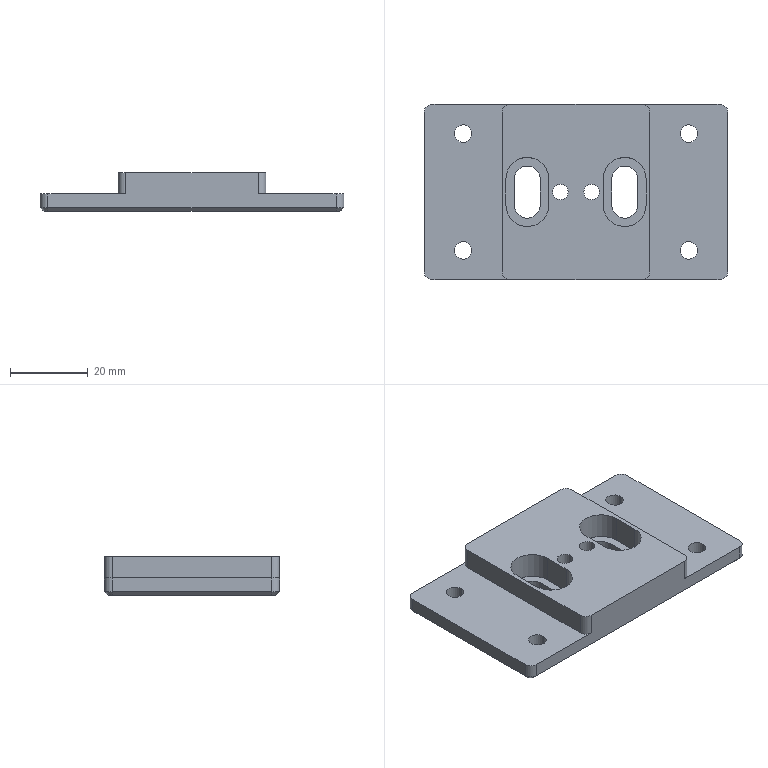Part | 1 solid | 56 faces | box 78 x 45 x 10 mm | volume 21692 mm3 | cylinder 28 | plane 24 | cone 4 | commonest cylinder face diameters 4 x12 4.5 x8 6.6 x4 11 x4